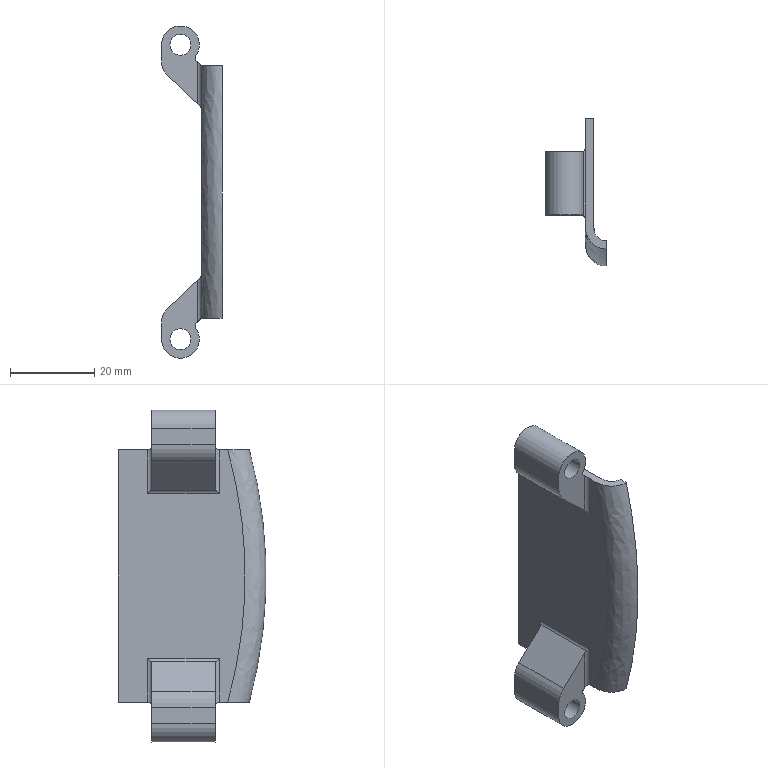Part | SolidWorks | features ICE 4, Fillet 2, Sweep 2, MirrorPattern 1 | 1 solid | 36 faces | box 14.5 x 35.129 x 79 mm | volume 7419 mm3 | cylinder 18 | plane 16 | spline 2 | commonest cylinder face diameters 2 x8 5 x4 9 x4 10 x2